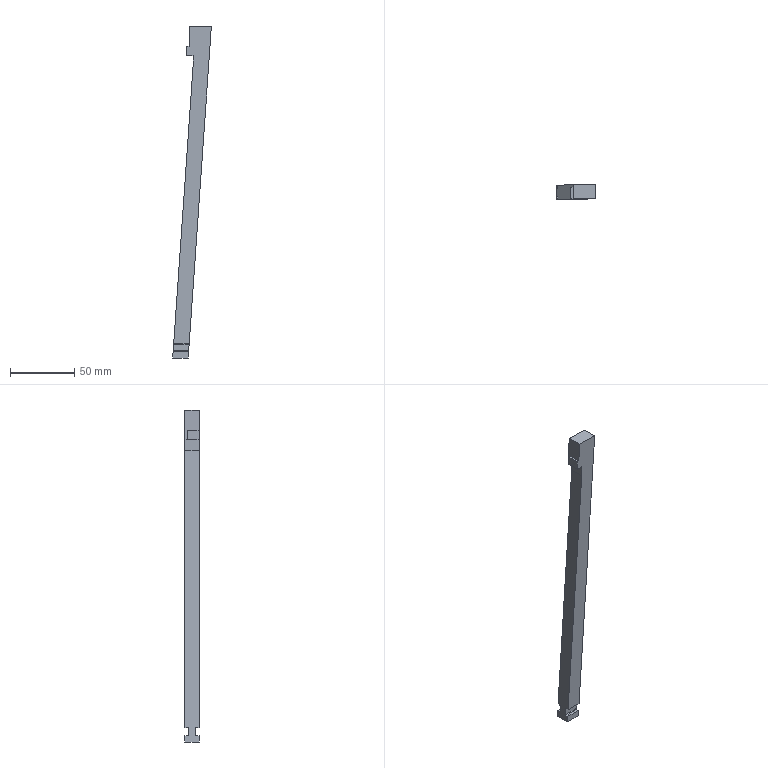Part | Creo | 1 solid | 113 faces | box 29.988 x 11 x 257.478 mm | volume 34897 mm3 | other 67 | plane 39 | cylinder 7 | commonest cylinder face diameters 1 x4 1.867 x2 29.451 x1